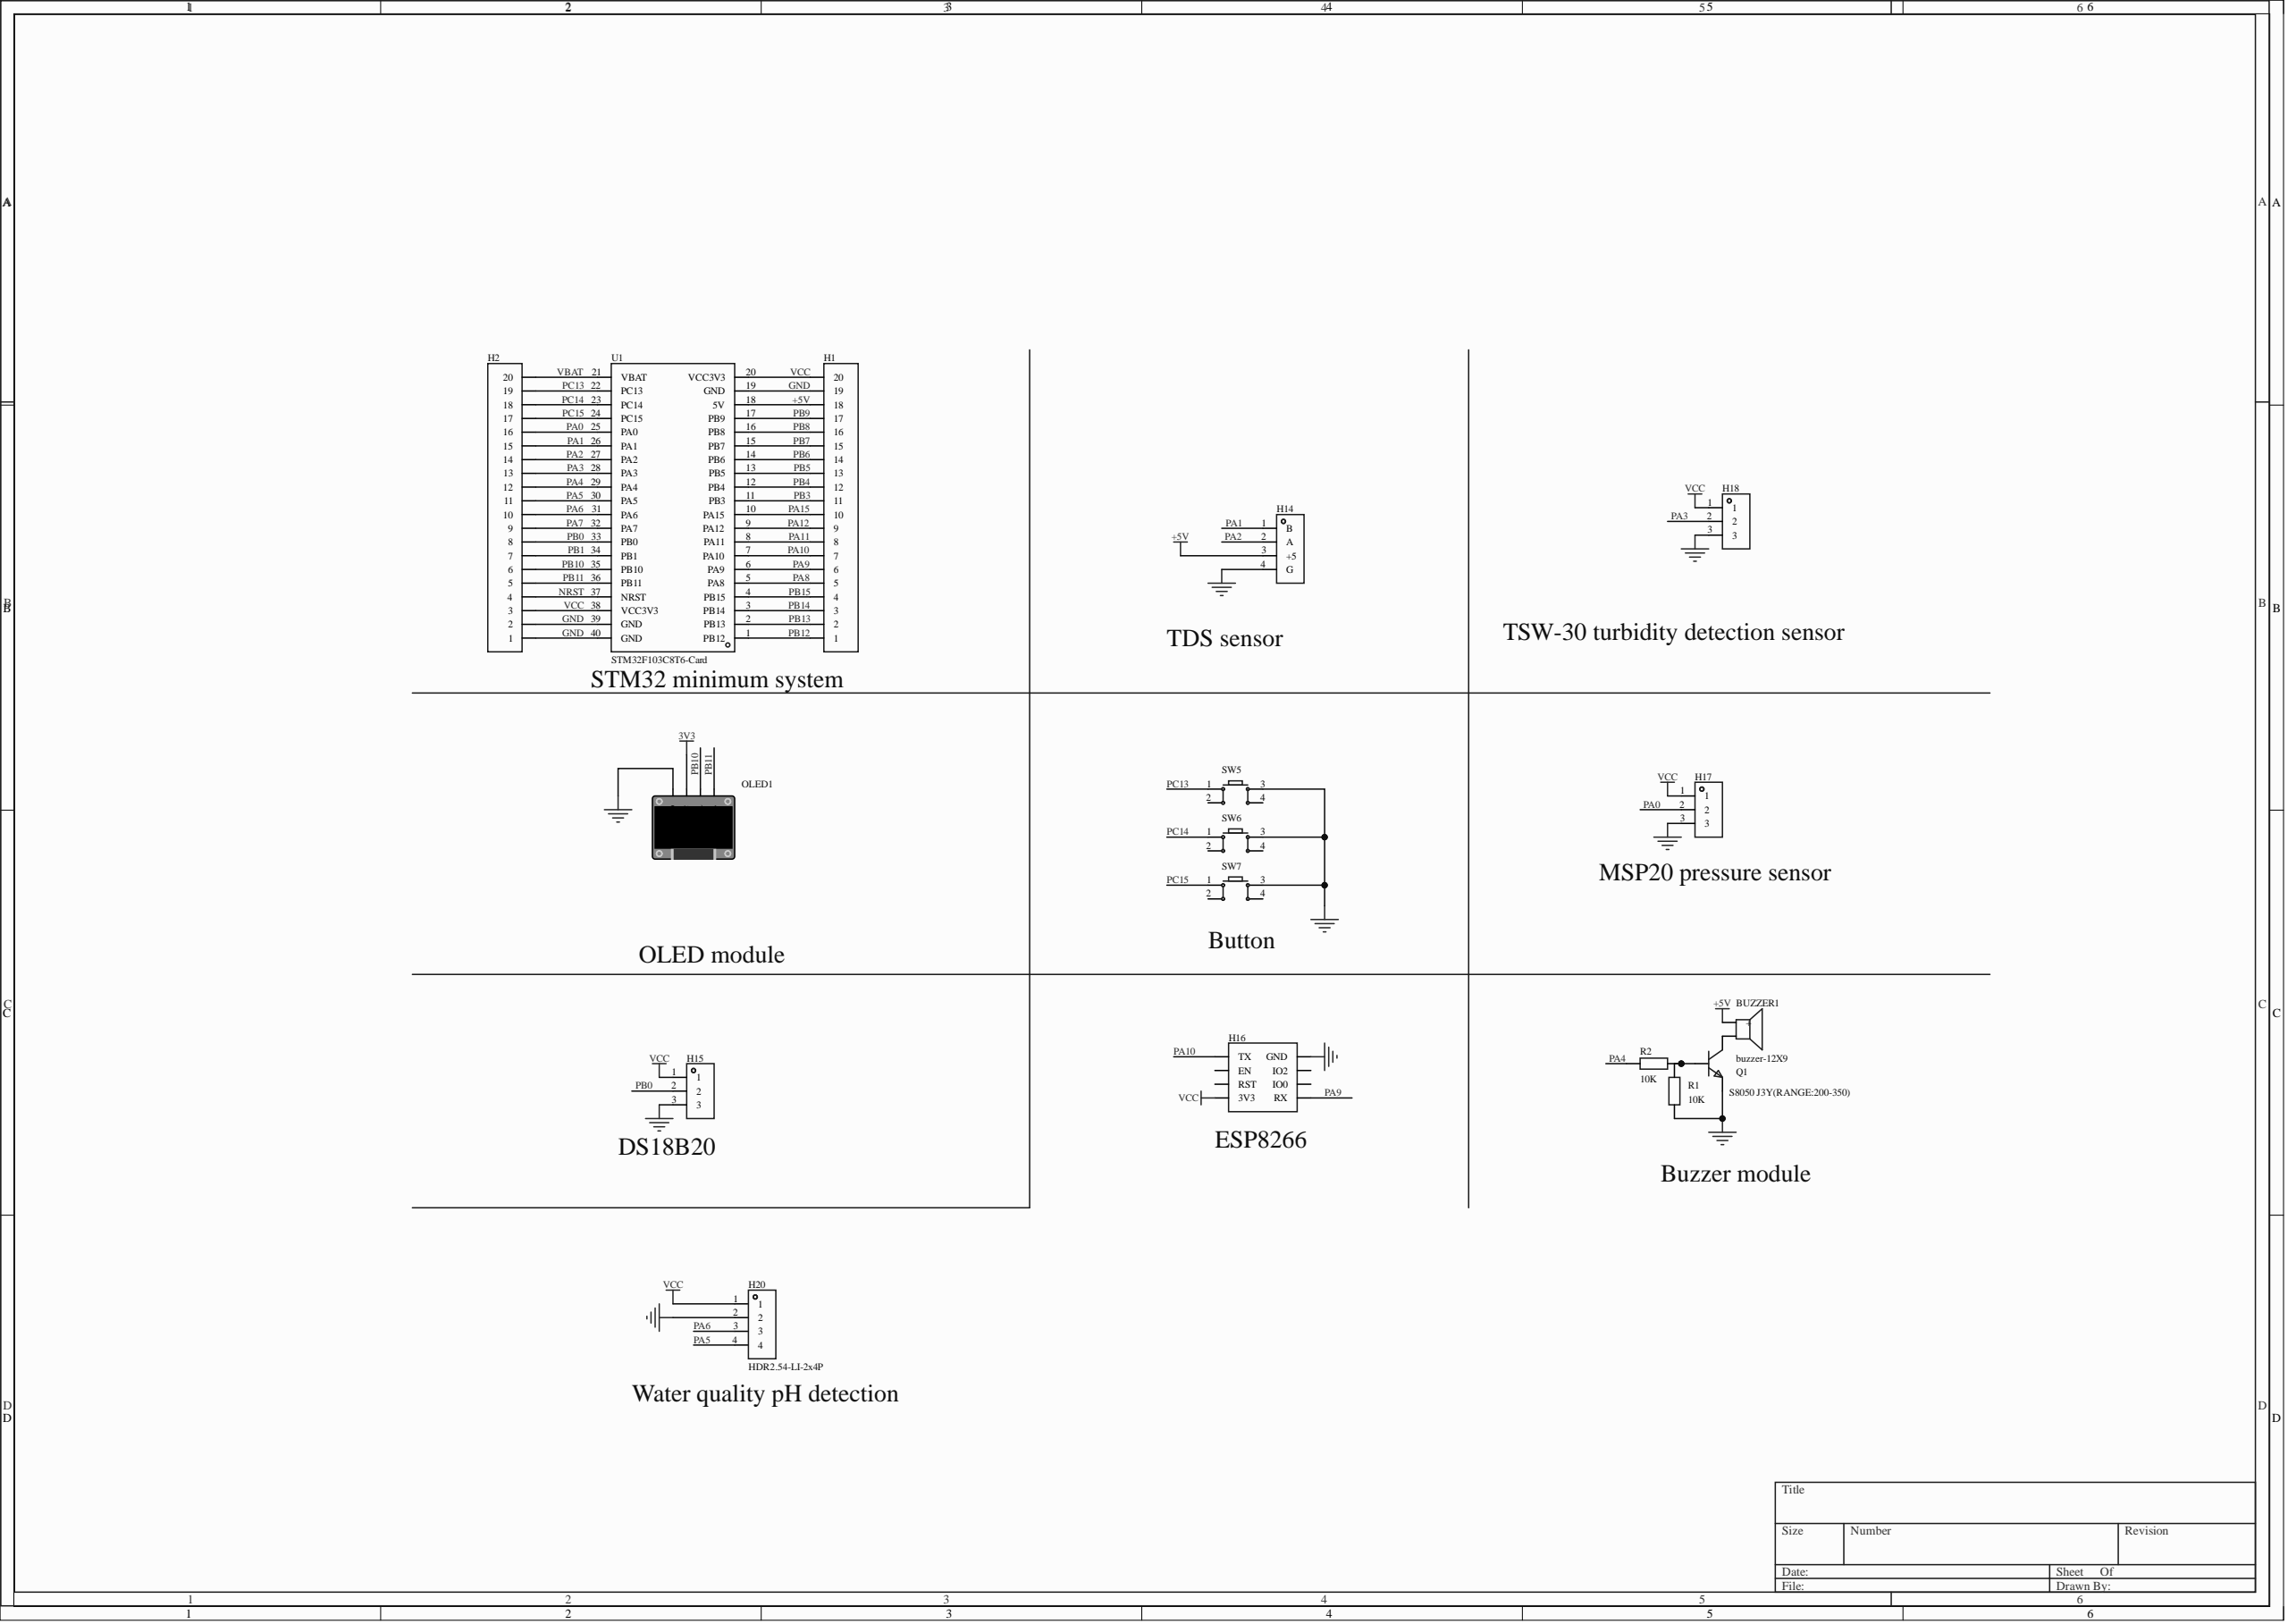Circuit board | Altium Designer | 17 parts | 39 nets
Bill of materials:
Comment,Description,Designator,Footprint,LibRef,Quantity
"buzzer-12X9","","BUZZER1","BUZ-TH_BD12.0-P7.60-D0.6-FD","buzzer-12X9","1"
"","","H1, H2","HDR-TH_20P-P2.54-V-F","HDR-F_2.54_1x20P","2"
"","","H14","HDR-TH_4P-P2.54-V-F","HDR-F_2.54_1x4P","1"
"","","H15, H17, H18","HDR-TH_3P-P2.54-V-F","HDR-F_2.54_1x3P","3"
"","","H16","HDR-TH_8P-P2.54-V-F-R2-C4-S2.54-1","HDR-F_2.54_2x4","1"
"HDR2.54-LI-2x4P","","H20","HDR-TH_4P-P2.54-V-M","HDR2.54-LI-2x4P","1"
"","","OLED1","0.96OLED_4P","0.96OLED模块_4P","1"
"S8050 J3Y(RANGE:200-350)","Transistor type:NPN; Collector current (Ic):500mA; Collector-emitter breakdown voltage (Vceo):25V; Power dissipation (Pd):300mW; DC current gain (hFE):200@500mA,1V;","Q1","SOT-23-3_L3.0-W1.7-P0.95-LS2.9-BR","S8050 J3Y(RANGE:200-350)","1"
"10K","","R1, R2","R0603","Res_0603","2"
"","","SW5, SW6, SW7","SW-TH_4P-L6.0-W6.0-P4.50-LS6.5","Key_TH_6x6x6","3"
"STM32F103C8T6-Card","","U1","CONN-TH_L53.3-W22.9_STM32F103C8T6-CARD","STM32F103C8T6-Card","1"
Netlist (Protel format):
[
BUZZER1
BUZ-TH_BD12.0-P7.60-D0.6-FD
buzzer-12X9



]
[
H1
HDR-TH_20P-P2.54-V-F




]
[
H2
HDR-TH_20P-P2.54-V-F




]
[
H14
HDR-TH_4P-P2.54-V-F




]
[
H15
HDR-TH_3P-P2.54-V-F




]
[
H16
HDR-TH_8P-P2.54-V-F-R2-C4-S2.54-1




]
[
H17
HDR-TH_3P-P2.54-V-F




]
[
H18
HDR-TH_3P-P2.54-V-F




]
[
H20
HDR-TH_4P-P2.54-V-M
HDR2.54-LI-2x4P



]
[
OLED1
0.96OLED_4P




]
[
Q1
SOT-23-3_L3.0-W1.7-P0.95-LS2.9-BR
S8050 J3Y(RANGE:200-350)



]
[
R1
R0603
10K



]
[
R2
R0603
10K



]
[
SW5
SW-TH_4P-L6.0-W6.0-P4.50-LS6.5




]
[
SW6
SW-TH_4P-L6.0-W6.0-P4.50-LS6.5




]
[
SW7
SW-TH_4P-L6.0-W6.0-P4.50-LS6.5




]
[
U1
CONN-TH_L53.3-W22.9_STM32F103C8T6-CARD
STM32F103C8T6-Card



]
(
VCC
H1-20
H2-3
H15-1
H16-7
H17-1
H18-1
H20-1
U1-20
U1-38
)
(
VBAT
H2-20
U1-21
)
(
PC15
H2-17
SW7-1
U1-24
)
(
PC14
H2-18
SW6-1
U1-23
)
(
PC13
H2-19
SW5-1
U1-22
)
(
PB15
H1-4
U1-4
)
(
PB14
H1-3
U1-3
)
(
PB13
H1-2
U1-2
)
(
PB12
H1-1
U1-1
)
(
PB11
H2-5
OLED1-4
U1-36
)
(
PB10
H2-6
OLED1-3
U1-35
)
(
PB9
H1-17
U1-17
)
(
PB8
H1-16
U1-16
)
(
PB7
H1-15
U1-15
)
(
PB6
H1-14
U1-14
)
(
PB5
H1-13
U1-13
)
(
PB4
H1-12
U1-12
)
(
PB3
H1-11
U1-11
)
(
PB1
H2-7
U1-34
)
(
PB0
H2-8
H15-2
U1-33
)
(
PA15
H1-10
U1-10
)
(
PA12
H1-9
U1-9
)
(
PA11
H1-8
U1-8
)
(
PA10
H1-7
H16-1
U1-7
)
(
PA9
H1-6
H16-8
U1-6
)
(
PA8
H1-5
U1-5
)
(
PA7
H2-9
U1-32
)
(
PA6
H2-10
H20-3
U1-31
)
(
PA5
H2-11
H20-4
U1-30
)
(
PA4
H2-12
R2-2
U1-29
)
(
PA3
H2-13
H18-2
U1-28
)
(
PA2
H2-14
H14-2
U1-27
)
(
PA1
H2-15
H14-1
U1-26
)
(
PA0
H2-16
H17-2
U1-25
)
(
NRST
H2-4
U1-37
)
(
NetQ1_1
Q1-1
R1-2
R2-1
)
(
NetBUZZER1_2
BUZZER1-2
Q1-3
)
(
GND
H1-19
H2-1
H2-2
H14-4
H15-3
H16-2
H17-3
H18-3
H20-2
OLED1-1
Q1-2
R1-1
SW5-3
SW6-3
SW7-3
U1-19
U1-39
U1-40
)
(
+5V
BUZZER1-1
H1-18
H14-3
U1-18
)